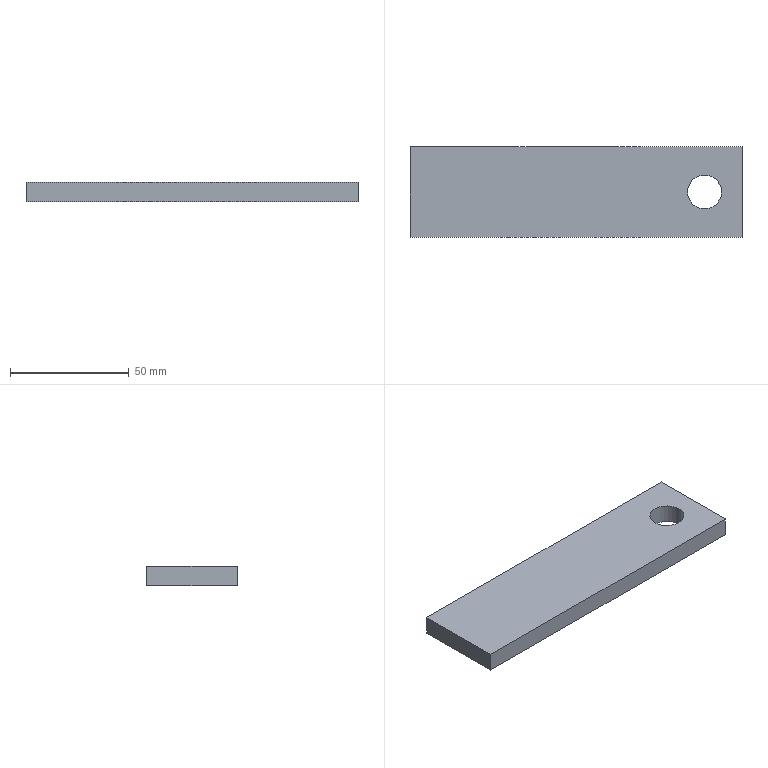Part | SolidWorks | features Extrusion 1 | 1 solid | 8 faces | box 139.7 x 38.1 x 8 mm | volume 41300 mm3 | plane 6 | cylinder 2 | commonest cylinder face diameters 14.275 x2
STEP:
#1=CARTESIAN_POINT('',(-7.137,0.,4.));
#2=VERTEX_POINT('',#1);
#3=CARTESIAN_POINT('',(7.137,0.,4.));
#4=VERTEX_POINT('',#3);
#5=CARTESIAN_POINT('',(0.,0.,4.));
#6=DIRECTION('',(0.,0.,1.));
#7=DIRECTION('',(1.,0.,0.));
#8=AXIS2_PLACEMENT_3D('',#5,#6,#7);
#9=CIRCLE('',#8,7.137);
#10=EDGE_CURVE('',#2,#4,#9,.T.);
#11=ORIENTED_EDGE('',*,*,#10,.T.);
#12=CARTESIAN_POINT('',(7.137,0.,-4.));
#13=VERTEX_POINT('',#12);
#14=CARTESIAN_POINT('',(7.137,0.,4.));
#15=DIRECTION('',(0.,0.,-1.));
#16=VECTOR('',#15,1000.);
#17=LINE('',#14,#16);
#18=EDGE_CURVE('',#4,#13,#17,.T.);
#19=ORIENTED_EDGE('',*,*,#18,.T.);
#20=CARTESIAN_POINT('',(-7.137,0.,-4.));
#21=VERTEX_POINT('',#20);
#22=CARTESIAN_POINT('',(0.,0.,-4.));
#23=DIRECTION('',(0.,0.,1.));
#24=DIRECTION('',(1.,0.,0.));
#25=AXIS2_PLACEMENT_3D('',#22,#23,#24);
#26=CIRCLE('',#25,7.137);
#27=EDGE_CURVE('',#21,#13,#26,.T.);
#28=ORIENTED_EDGE('',*,*,#27,.F.);
#29=CARTESIAN_POINT('',(-7.137,0.,4.));
#30=DIRECTION('',(0.,0.,-1.));
#31=VECTOR('',#30,1000.);
#32=LINE('',#29,#31);
#33=EDGE_CURVE('',#2,#21,#32,.T.);
#34=ORIENTED_EDGE('',*,*,#33,.F.);
#35=EDGE_LOOP('',(#11,#19,#28,#34));
#36=FACE_OUTER_BOUND('',#35,.T.);
#37=CARTESIAN_POINT('',(0.,0.,4.));
#38=DIRECTION('',(0.,0.,-1.));
#39=DIRECTION('',(-1.,0.,0.));
#40=AXIS2_PLACEMENT_3D('',#37,#38,#39);
#41=CYLINDRICAL_SURFACE('',#40,7.137);
#42=ADVANCED_FACE('',(#36),#41,.F.);
#43=CARTESIAN_POINT('',(-123.952,19.05,4.));
#44=VERTEX_POINT('',#43);
#45=CARTESIAN_POINT('',(-123.952,-19.05,4.));
#46=VERTEX_POINT('',#45);
#47=CARTESIAN_POINT('',(-123.952,19.05,4.));
#48=DIRECTION('',(0.,-1.,0.));
#49=VECTOR('',#48,1000.);
#50=LINE('',#47,#49);
#51=EDGE_CURVE('',#44,#46,#50,.T.);
#52=ORIENTED_EDGE('',*,*,#51,.T.);
#53=CARTESIAN_POINT('',(15.748,-19.05,4.));
#54=VERTEX_POINT('',#53);
#55=CARTESIAN_POINT('',(-123.952,-19.05,4.));
#56=DIRECTION('',(1.,0.,0.));
#57=VECTOR('',#56,1000.);
#58=LINE('',#55,#57);
#59=EDGE_CURVE('',#46,#54,#58,.T.);
#60=ORIENTED_EDGE('',*,*,#59,.T.);
#61=CARTESIAN_POINT('',(15.748,19.05,4.));
#62=VERTEX_POINT('',#61);
#63=CARTESIAN_POINT('',(15.748,19.05,4.));
#64=DIRECTION('',(0.,1.,0.));
#65=VECTOR('',#64,1000.);
#66=LINE('',#63,#65);
#67=EDGE_CURVE('',#54,#62,#66,.T.);
#68=ORIENTED_EDGE('',*,*,#67,.T.);
#69=CARTESIAN_POINT('',(-123.952,19.05,4.));
#70=DIRECTION('',(-1.,0.,0.));
#71=VECTOR('',#70,1000.);
#72=LINE('',#69,#71);
#73=EDGE_CURVE('',#62,#44,#72,.T.);
#74=ORIENTED_EDGE('',*,*,#73,.T.);
#75=EDGE_LOOP('',(#52,#60,#68,#74));
#76=FACE_OUTER_BOUND('',#75,.T.);
#77=ORIENTED_EDGE('',*,*,#10,.F.);
#78=CARTESIAN_POINT('',(0.,0.,4.));
#79=DIRECTION('',(0.,0.,1.));
#80=DIRECTION('',(1.,0.,0.));
#81=AXIS2_PLACEMENT_3D('',#78,#79,#80);
#82=CIRCLE('',#81,7.137);
#83=EDGE_CURVE('',#4,#2,#82,.T.);
#84=ORIENTED_EDGE('',*,*,#83,.F.);
#85=EDGE_LOOP('',(#77,#84));
#86=FACE_BOUND('',#85,.T.);
#87=CARTESIAN_POINT('',(0.,0.,4.));
#88=DIRECTION('',(0.,0.,1.));
#89=DIRECTION('',(1.,0.,0.));
#90=AXIS2_PLACEMENT_3D('',#87,#88,#89);
#91=PLANE('',#90);
#92=ADVANCED_FACE('',(#76,#86),#91,.T.);
#93=CARTESIAN_POINT('',(-123.952,19.05,-4.));
#94=VERTEX_POINT('',#93);
#95=CARTESIAN_POINT('',(-123.952,-19.05,-4.));
#96=VERTEX_POINT('',#95);
#97=CARTESIAN_POINT('',(-123.952,19.05,-4.));
#98=DIRECTION('',(0.,-1.,0.));
#99=VECTOR('',#98,1000.);
#100=LINE('',#97,#99);
#101=EDGE_CURVE('',#94,#96,#100,.T.);
#102=ORIENTED_EDGE('',*,*,#101,.F.);
#103=CARTESIAN_POINT('',(15.748,19.05,-4.));
#104=VERTEX_POINT('',#103);
#105=CARTESIAN_POINT('',(-123.952,19.05,-4.));
#106=DIRECTION('',(-1.,0.,0.));
#107=VECTOR('',#106,1000.);
#108=LINE('',#105,#107);
#109=EDGE_CURVE('',#104,#94,#108,.T.);
#110=ORIENTED_EDGE('',*,*,#109,.F.);
#111=CARTESIAN_POINT('',(15.748,-19.05,-4.));
#112=VERTEX_POINT('',#111);
#113=CARTESIAN_POINT('',(15.748,19.05,-4.));
#114=DIRECTION('',(0.,1.,0.));
#115=VECTOR('',#114,1000.);
#116=LINE('',#113,#115);
#117=EDGE_CURVE('',#112,#104,#116,.T.);
#118=ORIENTED_EDGE('',*,*,#117,.F.);
#119=CARTESIAN_POINT('',(-123.952,-19.05,-4.));
#120=DIRECTION('',(1.,0.,0.));
#121=VECTOR('',#120,1000.);
#122=LINE('',#119,#121);
#123=EDGE_CURVE('',#96,#112,#122,.T.);
#124=ORIENTED_EDGE('',*,*,#123,.F.);
#125=EDGE_LOOP('',(#102,#110,#118,#124));
#126=FACE_OUTER_BOUND('',#125,.T.);
#127=ORIENTED_EDGE('',*,*,#27,.T.);
#128=CARTESIAN_POINT('',(0.,0.,-4.));
#129=DIRECTION('',(0.,0.,1.));
#130=DIRECTION('',(1.,0.,0.));
#131=AXIS2_PLACEMENT_3D('',#128,#129,#130);
#132=CIRCLE('',#131,7.137);
#133=EDGE_CURVE('',#13,#21,#132,.T.);
#134=ORIENTED_EDGE('',*,*,#133,.T.);
#135=EDGE_LOOP('',(#127,#134));
#136=FACE_BOUND('',#135,.T.);
#137=CARTESIAN_POINT('',(0.,0.,-4.));
#138=DIRECTION('',(0.,0.,1.));
#139=DIRECTION('',(1.,0.,0.));
#140=AXIS2_PLACEMENT_3D('',#137,#138,#139);
#141=PLANE('',#140);
#142=ADVANCED_FACE('',(#126,#136),#141,.F.);
#143=ORIENTED_EDGE('',*,*,#101,.T.);
#144=CARTESIAN_POINT('',(-123.952,-19.05,4.));
#145=DIRECTION('',(0.,0.,-1.));
#146=VECTOR('',#145,1000.);
#147=LINE('',#144,#146);
#148=EDGE_CURVE('',#46,#96,#147,.T.);
#149=ORIENTED_EDGE('',*,*,#148,.F.);
#150=ORIENTED_EDGE('',*,*,#51,.F.);
#151=CARTESIAN_POINT('',(-123.952,19.05,4.));
#152=DIRECTION('',(0.,0.,-1.));
#153=VECTOR('',#152,1000.);
#154=LINE('',#151,#153);
#155=EDGE_CURVE('',#44,#94,#154,.T.);
#156=ORIENTED_EDGE('',*,*,#155,.T.);
#157=EDGE_LOOP('',(#143,#149,#150,#156));
#158=FACE_OUTER_BOUND('',#157,.T.);
#159=CARTESIAN_POINT('',(-123.952,19.05,4.));
#160=DIRECTION('',(1.,0.,0.));
#161=DIRECTION('',(0.,1.,0.));
#162=AXIS2_PLACEMENT_3D('',#159,#160,#161);
#163=PLANE('',#162);
#164=ADVANCED_FACE('',(#158),#163,.F.);
#165=ORIENTED_EDGE('',*,*,#123,.T.);
#166=CARTESIAN_POINT('',(15.748,-19.05,4.));
#167=DIRECTION('',(0.,0.,-1.));
#168=VECTOR('',#167,1000.);
#169=LINE('',#166,#168);
#170=EDGE_CURVE('',#54,#112,#169,.T.);
#171=ORIENTED_EDGE('',*,*,#170,.F.);
#172=ORIENTED_EDGE('',*,*,#59,.F.);
#173=ORIENTED_EDGE('',*,*,#148,.T.);
#174=EDGE_LOOP('',(#165,#171,#172,#173));
#175=FACE_OUTER_BOUND('',#174,.T.);
#176=CARTESIAN_POINT('',(-123.952,-19.05,4.));
#177=DIRECTION('',(0.,1.,0.));
#178=DIRECTION('',(-1.,0.,0.));
#179=AXIS2_PLACEMENT_3D('',#176,#177,#178);
#180=PLANE('',#179);
#181=ADVANCED_FACE('',(#175),#180,.F.);
#182=ORIENTED_EDGE('',*,*,#117,.T.);
#183=CARTESIAN_POINT('',(15.748,19.05,4.));
#184=DIRECTION('',(0.,0.,-1.));
#185=VECTOR('',#184,1000.);
#186=LINE('',#183,#185);
#187=EDGE_CURVE('',#62,#104,#186,.T.);
#188=ORIENTED_EDGE('',*,*,#187,.F.);
#189=ORIENTED_EDGE('',*,*,#67,.F.);
#190=ORIENTED_EDGE('',*,*,#170,.T.);
#191=EDGE_LOOP('',(#182,#188,#189,#190));
#192=FACE_OUTER_BOUND('',#191,.T.);
#193=CARTESIAN_POINT('',(15.748,19.05,4.));
#194=DIRECTION('',(-1.,0.,0.));
#195=DIRECTION('',(0.,0.,1.));
#196=AXIS2_PLACEMENT_3D('',#193,#194,#195);
#197=PLANE('',#196);
#198=ADVANCED_FACE('',(#192),#197,.F.);
#199=ORIENTED_EDGE('',*,*,#109,.T.);
#200=ORIENTED_EDGE('',*,*,#155,.F.);
#201=ORIENTED_EDGE('',*,*,#73,.F.);
#202=ORIENTED_EDGE('',*,*,#187,.T.);
#203=EDGE_LOOP('',(#199,#200,#201,#202));
#204=FACE_OUTER_BOUND('',#203,.T.);
#205=CARTESIAN_POINT('',(-123.952,19.05,4.));
#206=DIRECTION('',(0.,-1.,0.));
#207=DIRECTION('',(0.,0.,-1.));
#208=AXIS2_PLACEMENT_3D('',#205,#206,#207);
#209=PLANE('',#208);
#210=ADVANCED_FACE('',(#204),#209,.F.);
#211=ORIENTED_EDGE('',*,*,#18,.F.);
#212=ORIENTED_EDGE('',*,*,#83,.T.);
#213=ORIENTED_EDGE('',*,*,#33,.T.);
#214=ORIENTED_EDGE('',*,*,#133,.F.);
#215=EDGE_LOOP('',(#211,#212,#213,#214));
#216=FACE_OUTER_BOUND('',#215,.T.);
#217=CARTESIAN_POINT('',(0.,0.,4.));
#218=DIRECTION('',(0.,0.,-1.));
#219=DIRECTION('',(-1.,0.,0.));
#220=AXIS2_PLACEMENT_3D('',#217,#218,#219);
#221=CYLINDRICAL_SURFACE('',#220,7.137);
#222=ADVANCED_FACE('',(#216),#221,.F.);
#223=CLOSED_SHELL('',(#42,#92,#142,#164,#181,#198,#210,#222));
#224=MANIFOLD_SOLID_BREP('',#223);
#225=CARTESIAN_POINT('',(0.,0.,0.));
#226=DIRECTION('',(0.,0.,1.));
#227=DIRECTION('',(1.,0.,0.));
#228=AXIS2_PLACEMENT_3D('',#225,#226,#227);
#229=(LENGTH_UNIT()NAMED_UNIT(*)SI_UNIT(.MILLI.,.METRE.));
#230=UNCERTAINTY_MEASURE_WITH_UNIT(LENGTH_MEASURE(0.00001),#229,'','');
#231=(NAMED_UNIT(*)PLANE_ANGLE_UNIT()SI_UNIT($,.RADIAN.));
#232=(NAMED_UNIT(*)SI_UNIT($,.STERADIAN.)SOLID_ANGLE_UNIT());
#233=(GEOMETRIC_REPRESENTATION_CONTEXT(3)GLOBAL_UNCERTAINTY_ASSIGNED_CONTEXT((#230))GLOBAL_UNIT_ASSIGNED_CONTEXT((#229,#231,#232))REPRESENTATION_CONTEXT('',''));
#234=ADVANCED_BREP_SHAPE_REPRESENTATION('',(#224,#228),#233);